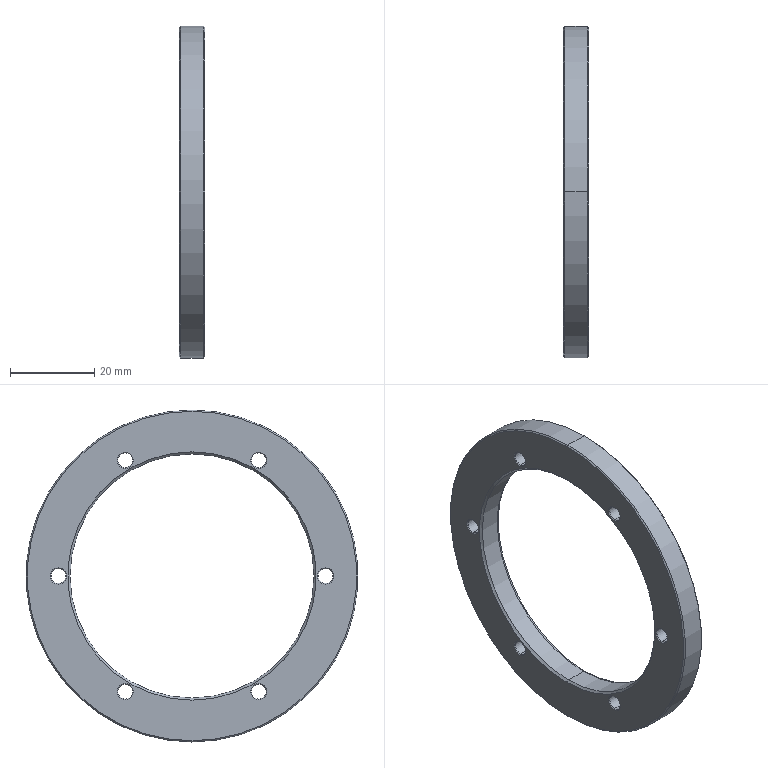Part | SolidWorks | features BaseBody 1 | 1 solid | 53 faces | box 6 x 78.9 x 78.9 mm | volume 13059 mm3 | cone 32 | cylinder 16 | plane 3 | torus 2 | commonest cylinder face diameters 3.5 x12 58 x2 78.9 x2
STEP:
#1=CARTESIAN_POINT('',(5.8,31.75,1.75));
#2=VERTEX_POINT('',#1);
#3=CARTESIAN_POINT('',(5.8,31.75,-1.75));
#4=VERTEX_POINT('',#3);
#5=CARTESIAN_POINT('',(5.8,31.75,0.));
#6=DIRECTION('',(1.,0.,0.));
#7=DIRECTION('',(0.,0.,1.));
#8=AXIS2_PLACEMENT_3D('',#5,#6,#7);
#9=CIRCLE('',#8,1.75);
#10=EDGE_CURVE('',#2,#4,#9,.T.);
#11=ORIENTED_EDGE('',*,*,#10,.F.);
#12=CARTESIAN_POINT('',(6.,31.75,1.95));
#13=VERTEX_POINT('',#12);
#14=CARTESIAN_POINT('',(6.,31.75,1.95));
#15=DIRECTION('',(0.7071,0.,0.7071));
#16=VECTOR('',#15,1000.);
#17=LINE('',#14,#16);
#18=EDGE_CURVE('',#2,#13,#17,.T.);
#19=ORIENTED_EDGE('',*,*,#18,.T.);
#20=CARTESIAN_POINT('',(6.,31.75,-1.95));
#21=VERTEX_POINT('',#20);
#22=CARTESIAN_POINT('',(6.,31.75,0.));
#23=DIRECTION('',(-1.,0.,0.));
#24=DIRECTION('',(0.,0.,1.));
#25=AXIS2_PLACEMENT_3D('',#22,#23,#24);
#26=CIRCLE('',#25,1.95);
#27=EDGE_CURVE('',#21,#13,#26,.T.);
#28=ORIENTED_EDGE('',*,*,#27,.F.);
#29=CARTESIAN_POINT('',(6.,31.75,-1.95));
#30=DIRECTION('',(0.7071,0.,-0.7071));
#31=VECTOR('',#30,1000.);
#32=LINE('',#29,#31);
#33=EDGE_CURVE('',#4,#21,#32,.T.);
#34=ORIENTED_EDGE('',*,*,#33,.F.);
#35=EDGE_LOOP('',(#11,#19,#28,#34));
#36=FACE_OUTER_BOUND('',#35,.T.);
#37=CARTESIAN_POINT('',(6.,31.75,0.));
#38=DIRECTION('',(1.,0.,0.));
#39=DIRECTION('',(0.,0.,-1.));
#40=AXIS2_PLACEMENT_3D('',#37,#38,#39);
#41=CONICAL_SURFACE('',#40,1.95,0.7854);
#42=ADVANCED_FACE('',(#36),#41,.F.);
#43=CARTESIAN_POINT('',(0.2,31.75,-1.75));
#44=VERTEX_POINT('',#43);
#45=CARTESIAN_POINT('',(0.2,31.75,1.75));
#46=VERTEX_POINT('',#45);
#47=CARTESIAN_POINT('',(0.2,31.75,0.));
#48=DIRECTION('',(-1.,0.,0.));
#49=DIRECTION('',(0.,0.,-1.));
#50=AXIS2_PLACEMENT_3D('',#47,#48,#49);
#51=CIRCLE('',#50,1.75);
#52=EDGE_CURVE('',#44,#46,#51,.T.);
#53=ORIENTED_EDGE('',*,*,#52,.F.);
#54=CARTESIAN_POINT('',(0.,31.75,-1.95));
#55=VERTEX_POINT('',#54);
#56=CARTESIAN_POINT('',(0.2,31.75,-1.75));
#57=DIRECTION('',(-0.7071,0.,-0.7071));
#58=VECTOR('',#57,1000.);
#59=LINE('',#56,#58);
#60=EDGE_CURVE('',#44,#55,#59,.T.);
#61=ORIENTED_EDGE('',*,*,#60,.T.);
#62=CARTESIAN_POINT('',(0.,31.75,1.95));
#63=VERTEX_POINT('',#62);
#64=CARTESIAN_POINT('',(0.,31.75,0.));
#65=DIRECTION('',(1.,0.,0.));
#66=DIRECTION('',(0.,0.,-1.));
#67=AXIS2_PLACEMENT_3D('',#64,#65,#66);
#68=CIRCLE('',#67,1.95);
#69=EDGE_CURVE('',#63,#55,#68,.T.);
#70=ORIENTED_EDGE('',*,*,#69,.F.);
#71=CARTESIAN_POINT('',(0.2,31.75,1.75));
#72=DIRECTION('',(-0.7071,0.,0.7071));
#73=VECTOR('',#72,1000.);
#74=LINE('',#71,#73);
#75=EDGE_CURVE('',#46,#63,#74,.T.);
#76=ORIENTED_EDGE('',*,*,#75,.F.);
#77=EDGE_LOOP('',(#53,#61,#70,#76));
#78=FACE_OUTER_BOUND('',#77,.T.);
#79=CARTESIAN_POINT('',(0.2,31.75,0.));
#80=DIRECTION('',(-1.,0.,0.));
#81=DIRECTION('',(0.,0.,1.));
#82=AXIS2_PLACEMENT_3D('',#79,#80,#81);
#83=CONICAL_SURFACE('',#82,1.75,0.7854);
#84=ADVANCED_FACE('',(#78),#83,.F.);
#85=CARTESIAN_POINT('',(5.8,15.875,-25.746));
#86=VERTEX_POINT('',#85);
#87=CARTESIAN_POINT('',(5.8,15.875,-29.246));
#88=VERTEX_POINT('',#87);
#89=CARTESIAN_POINT('',(5.8,15.875,-27.496));
#90=DIRECTION('',(1.,0.,0.));
#91=DIRECTION('',(0.,0.,1.));
#92=AXIS2_PLACEMENT_3D('',#89,#90,#91);
#93=CIRCLE('',#92,1.75);
#94=EDGE_CURVE('',#86,#88,#93,.T.);
#95=ORIENTED_EDGE('',*,*,#94,.F.);
#96=CARTESIAN_POINT('',(6.,15.875,-25.546));
#97=VERTEX_POINT('',#96);
#98=CARTESIAN_POINT('',(6.,15.875,-25.546));
#99=DIRECTION('',(0.7071,0.,0.7071));
#100=VECTOR('',#99,1000.);
#101=LINE('',#98,#100);
#102=EDGE_CURVE('',#86,#97,#101,.T.);
#103=ORIENTED_EDGE('',*,*,#102,.T.);
#104=CARTESIAN_POINT('',(6.,15.875,-29.446));
#105=VERTEX_POINT('',#104);
#106=CARTESIAN_POINT('',(6.,15.875,-27.496));
#107=DIRECTION('',(-1.,0.,0.));
#108=DIRECTION('',(0.,0.,1.));
#109=AXIS2_PLACEMENT_3D('',#106,#107,#108);
#110=CIRCLE('',#109,1.95);
#111=EDGE_CURVE('',#105,#97,#110,.T.);
#112=ORIENTED_EDGE('',*,*,#111,.F.);
#113=CARTESIAN_POINT('',(6.,15.875,-29.446));
#114=DIRECTION('',(0.7071,0.,-0.7071));
#115=VECTOR('',#114,1000.);
#116=LINE('',#113,#115);
#117=EDGE_CURVE('',#88,#105,#116,.T.);
#118=ORIENTED_EDGE('',*,*,#117,.F.);
#119=EDGE_LOOP('',(#95,#103,#112,#118));
#120=FACE_OUTER_BOUND('',#119,.T.);
#121=CARTESIAN_POINT('',(6.,15.875,-27.496));
#122=DIRECTION('',(1.,0.,0.));
#123=DIRECTION('',(0.,0.,-1.));
#124=AXIS2_PLACEMENT_3D('',#121,#122,#123);
#125=CONICAL_SURFACE('',#124,1.95,0.7854);
#126=ADVANCED_FACE('',(#120),#125,.F.);
#127=CARTESIAN_POINT('',(0.2,15.875,-29.246));
#128=VERTEX_POINT('',#127);
#129=CARTESIAN_POINT('',(0.2,15.875,-25.746));
#130=VERTEX_POINT('',#129);
#131=CARTESIAN_POINT('',(0.2,15.875,-27.496));
#132=DIRECTION('',(-1.,0.,0.));
#133=DIRECTION('',(0.,0.,-1.));
#134=AXIS2_PLACEMENT_3D('',#131,#132,#133);
#135=CIRCLE('',#134,1.75);
#136=EDGE_CURVE('',#128,#130,#135,.T.);
#137=ORIENTED_EDGE('',*,*,#136,.F.);
#138=CARTESIAN_POINT('',(0.,15.875,-29.446));
#139=VERTEX_POINT('',#138);
#140=CARTESIAN_POINT('',(0.2,15.875,-29.246));
#141=DIRECTION('',(-0.7071,0.,-0.7071));
#142=VECTOR('',#141,1000.);
#143=LINE('',#140,#142);
#144=EDGE_CURVE('',#128,#139,#143,.T.);
#145=ORIENTED_EDGE('',*,*,#144,.T.);
#146=CARTESIAN_POINT('',(0.,15.875,-25.546));
#147=VERTEX_POINT('',#146);
#148=CARTESIAN_POINT('',(0.,15.875,-27.496));
#149=DIRECTION('',(1.,0.,0.));
#150=DIRECTION('',(0.,0.,-1.));
#151=AXIS2_PLACEMENT_3D('',#148,#149,#150);
#152=CIRCLE('',#151,1.95);
#153=EDGE_CURVE('',#147,#139,#152,.T.);
#154=ORIENTED_EDGE('',*,*,#153,.F.);
#155=CARTESIAN_POINT('',(0.2,15.875,-25.746));
#156=DIRECTION('',(-0.7071,0.,0.7071));
#157=VECTOR('',#156,1000.);
#158=LINE('',#155,#157);
#159=EDGE_CURVE('',#130,#147,#158,.T.);
#160=ORIENTED_EDGE('',*,*,#159,.F.);
#161=EDGE_LOOP('',(#137,#145,#154,#160));
#162=FACE_OUTER_BOUND('',#161,.T.);
#163=CARTESIAN_POINT('',(0.2,15.875,-27.496));
#164=DIRECTION('',(-1.,0.,0.));
#165=DIRECTION('',(0.,0.,1.));
#166=AXIS2_PLACEMENT_3D('',#163,#164,#165);
#167=CONICAL_SURFACE('',#166,1.75,0.7854);
#168=ADVANCED_FACE('',(#162),#167,.F.);
#169=CARTESIAN_POINT('',(5.8,-15.875,-25.746));
#170=VERTEX_POINT('',#169);
#171=CARTESIAN_POINT('',(5.8,-15.875,-29.246));
#172=VERTEX_POINT('',#171);
#173=CARTESIAN_POINT('',(5.8,-15.875,-27.496));
#174=DIRECTION('',(1.,0.,0.));
#175=DIRECTION('',(0.,0.,1.));
#176=AXIS2_PLACEMENT_3D('',#173,#174,#175);
#177=CIRCLE('',#176,1.75);
#178=EDGE_CURVE('',#170,#172,#177,.T.);
#179=ORIENTED_EDGE('',*,*,#178,.F.);
#180=CARTESIAN_POINT('',(6.,-15.875,-25.546));
#181=VERTEX_POINT('',#180);
#182=CARTESIAN_POINT('',(6.,-15.875,-25.546));
#183=DIRECTION('',(0.7071,0.,0.7071));
#184=VECTOR('',#183,1000.);
#185=LINE('',#182,#184);
#186=EDGE_CURVE('',#170,#181,#185,.T.);
#187=ORIENTED_EDGE('',*,*,#186,.T.);
#188=CARTESIAN_POINT('',(6.,-15.875,-29.446));
#189=VERTEX_POINT('',#188);
#190=CARTESIAN_POINT('',(6.,-15.875,-27.496));
#191=DIRECTION('',(-1.,0.,0.));
#192=DIRECTION('',(0.,0.,1.));
#193=AXIS2_PLACEMENT_3D('',#190,#191,#192);
#194=CIRCLE('',#193,1.95);
#195=EDGE_CURVE('',#189,#181,#194,.T.);
#196=ORIENTED_EDGE('',*,*,#195,.F.);
#197=CARTESIAN_POINT('',(6.,-15.875,-29.446));
#198=DIRECTION('',(0.7071,0.,-0.7071));
#199=VECTOR('',#198,1000.);
#200=LINE('',#197,#199);
#201=EDGE_CURVE('',#172,#189,#200,.T.);
#202=ORIENTED_EDGE('',*,*,#201,.F.);
#203=EDGE_LOOP('',(#179,#187,#196,#202));
#204=FACE_OUTER_BOUND('',#203,.T.);
#205=CARTESIAN_POINT('',(6.,-15.875,-27.496));
#206=DIRECTION('',(1.,0.,0.));
#207=DIRECTION('',(0.,0.,-1.));
#208=AXIS2_PLACEMENT_3D('',#205,#206,#207);
#209=CONICAL_SURFACE('',#208,1.95,0.7854);
#210=ADVANCED_FACE('',(#204),#209,.F.);
#211=CARTESIAN_POINT('',(0.2,-15.875,-29.246));
#212=VERTEX_POINT('',#211);
#213=CARTESIAN_POINT('',(0.2,-15.875,-25.746));
#214=VERTEX_POINT('',#213);
#215=CARTESIAN_POINT('',(0.2,-15.875,-27.496));
#216=DIRECTION('',(-1.,0.,0.));
#217=DIRECTION('',(0.,0.,-1.));
#218=AXIS2_PLACEMENT_3D('',#215,#216,#217);
#219=CIRCLE('',#218,1.75);
#220=EDGE_CURVE('',#212,#214,#219,.T.);
#221=ORIENTED_EDGE('',*,*,#220,.F.);
#222=CARTESIAN_POINT('',(0.,-15.875,-29.446));
#223=VERTEX_POINT('',#222);
#224=CARTESIAN_POINT('',(0.2,-15.875,-29.246));
#225=DIRECTION('',(-0.7071,0.,-0.7071));
#226=VECTOR('',#225,1000.);
#227=LINE('',#224,#226);
#228=EDGE_CURVE('',#212,#223,#227,.T.);
#229=ORIENTED_EDGE('',*,*,#228,.T.);
#230=CARTESIAN_POINT('',(0.,-15.875,-25.546));
#231=VERTEX_POINT('',#230);
#232=CARTESIAN_POINT('',(0.,-15.875,-27.496));
#233=DIRECTION('',(1.,0.,0.));
#234=DIRECTION('',(0.,0.,-1.));
#235=AXIS2_PLACEMENT_3D('',#232,#233,#234);
#236=CIRCLE('',#235,1.95);
#237=EDGE_CURVE('',#231,#223,#236,.T.);
#238=ORIENTED_EDGE('',*,*,#237,.F.);
#239=CARTESIAN_POINT('',(0.2,-15.875,-25.746));
#240=DIRECTION('',(-0.7071,0.,0.7071));
#241=VECTOR('',#240,1000.);
#242=LINE('',#239,#241);
#243=EDGE_CURVE('',#214,#231,#242,.T.);
#244=ORIENTED_EDGE('',*,*,#243,.F.);
#245=EDGE_LOOP('',(#221,#229,#238,#244));
#246=FACE_OUTER_BOUND('',#245,.T.);
#247=CARTESIAN_POINT('',(0.2,-15.875,-27.496));
#248=DIRECTION('',(-1.,0.,0.));
#249=DIRECTION('',(0.,0.,1.));
#250=AXIS2_PLACEMENT_3D('',#247,#248,#249);
#251=CONICAL_SURFACE('',#250,1.75,0.7854);
#252=ADVANCED_FACE('',(#246),#251,.F.);
#253=CARTESIAN_POINT('',(5.8,-31.75,1.75));
#254=VERTEX_POINT('',#253);
#255=CARTESIAN_POINT('',(5.8,-31.75,-1.75));
#256=VERTEX_POINT('',#255);
#257=CARTESIAN_POINT('',(5.8,-31.75,0.));
#258=DIRECTION('',(1.,0.,0.));
#259=DIRECTION('',(0.,0.,1.));
#260=AXIS2_PLACEMENT_3D('',#257,#258,#259);
#261=CIRCLE('',#260,1.75);
#262=EDGE_CURVE('',#254,#256,#261,.T.);
#263=ORIENTED_EDGE('',*,*,#262,.F.);
#264=CARTESIAN_POINT('',(6.,-31.75,1.95));
#265=VERTEX_POINT('',#264);
#266=CARTESIAN_POINT('',(6.,-31.75,1.95));
#267=DIRECTION('',(0.7071,0.,0.7071));
#268=VECTOR('',#267,1000.);
#269=LINE('',#266,#268);
#270=EDGE_CURVE('',#254,#265,#269,.T.);
#271=ORIENTED_EDGE('',*,*,#270,.T.);
#272=CARTESIAN_POINT('',(6.,-31.75,-1.95));
#273=VERTEX_POINT('',#272);
#274=CARTESIAN_POINT('',(6.,-31.75,0.));
#275=DIRECTION('',(-1.,0.,0.));
#276=DIRECTION('',(0.,0.,1.));
#277=AXIS2_PLACEMENT_3D('',#274,#275,#276);
#278=CIRCLE('',#277,1.95);
#279=EDGE_CURVE('',#273,#265,#278,.T.);
#280=ORIENTED_EDGE('',*,*,#279,.F.);
#281=CARTESIAN_POINT('',(6.,-31.75,-1.95));
#282=DIRECTION('',(0.7071,0.,-0.7071));
#283=VECTOR('',#282,1000.);
#284=LINE('',#281,#283);
#285=EDGE_CURVE('',#256,#273,#284,.T.);
#286=ORIENTED_EDGE('',*,*,#285,.F.);
#287=EDGE_LOOP('',(#263,#271,#280,#286));
#288=FACE_OUTER_BOUND('',#287,.T.);
#289=CARTESIAN_POINT('',(6.,-31.75,0.));
#290=DIRECTION('',(1.,0.,0.));
#291=DIRECTION('',(0.,0.,-1.));
#292=AXIS2_PLACEMENT_3D('',#289,#290,#291);
#293=CONICAL_SURFACE('',#292,1.95,0.7854);
#294=ADVANCED_FACE('',(#288),#293,.F.);
#295=CARTESIAN_POINT('',(0.2,-31.75,-1.75));
#296=VERTEX_POINT('',#295);
#297=CARTESIAN_POINT('',(0.2,-31.75,1.75));
#298=VERTEX_POINT('',#297);
#299=CARTESIAN_POINT('',(0.2,-31.75,0.));
#300=DIRECTION('',(-1.,0.,0.));
#301=DIRECTION('',(0.,0.,-1.));
#302=AXIS2_PLACEMENT_3D('',#299,#300,#301);
#303=CIRCLE('',#302,1.75);
#304=EDGE_CURVE('',#296,#298,#303,.T.);
#305=ORIENTED_EDGE('',*,*,#304,.F.);
#306=CARTESIAN_POINT('',(0.,-31.75,-1.95));
#307=VERTEX_POINT('',#306);
#308=CARTESIAN_POINT('',(0.2,-31.75,-1.75));
#309=DIRECTION('',(-0.7071,0.,-0.7071));
#310=VECTOR('',#309,1000.);
#311=LINE('',#308,#310);
#312=EDGE_CURVE('',#296,#307,#311,.T.);
#313=ORIENTED_EDGE('',*,*,#312,.T.);
#314=CARTESIAN_POINT('',(0.,-31.75,1.95));
#315=VERTEX_POINT('',#314);
#316=CARTESIAN_POINT('',(0.,-31.75,0.));
#317=DIRECTION('',(1.,0.,0.));
#318=DIRECTION('',(0.,0.,-1.));
#319=AXIS2_PLACEMENT_3D('',#316,#317,#318);
#320=CIRCLE('',#319,1.95);
#321=EDGE_CURVE('',#315,#307,#320,.T.);
#322=ORIENTED_EDGE('',*,*,#321,.F.);
#323=CARTESIAN_POINT('',(0.2,-31.75,1.75));
#324=DIRECTION('',(-0.7071,0.,0.7071));
#325=VECTOR('',#324,1000.);
#326=LINE('',#323,#325);
#327=EDGE_CURVE('',#298,#315,#326,.T.);
#328=ORIENTED_EDGE('',*,*,#327,.F.);
#329=EDGE_LOOP('',(#305,#313,#322,#328));
#330=FACE_OUTER_BOUND('',#329,.T.);
#331=CARTESIAN_POINT('',(0.2,-31.75,0.));
#332=DIRECTION('',(-1.,0.,0.));
#333=DIRECTION('',(0.,0.,1.));
#334=AXIS2_PLACEMENT_3D('',#331,#332,#333);
#335=CONICAL_SURFACE('',#334,1.75,0.7854);
#336=ADVANCED_FACE('',(#330),#335,.F.);
#337=CARTESIAN_POINT('',(5.8,-15.875,29.246));
#338=VERTEX_POINT('',#337);
#339=CARTESIAN_POINT('',(5.8,-15.875,25.746));
#340=VERTEX_POINT('',#339);
#341=CARTESIAN_POINT('',(5.8,-15.875,27.496));
#342=DIRECTION('',(1.,0.,0.));
#343=DIRECTION('',(0.,0.,1.));
#344=AXIS2_PLACEMENT_3D('',#341,#342,#343);
#345=CIRCLE('',#344,1.75);
#346=EDGE_CURVE('',#338,#340,#345,.T.);
#347=ORIENTED_EDGE('',*,*,#346,.F.);
#348=CARTESIAN_POINT('',(6.,-15.875,29.446));
#349=VERTEX_POINT('',#348);
#350=CARTESIAN_POINT('',(6.,-15.875,29.446));
#351=DIRECTION('',(0.7071,0.,0.7071));
#352=VECTOR('',#351,1000.);
#353=LINE('',#350,#352);
#354=EDGE_CURVE('',#338,#349,#353,.T.);
#355=ORIENTED_EDGE('',*,*,#354,.T.);
#356=CARTESIAN_POINT('',(6.,-15.875,25.546));
#357=VERTEX_POINT('',#356);
#358=CARTESIAN_POINT('',(6.,-15.875,27.496));
#359=DIRECTION('',(-1.,0.,0.));
#360=DIRECTION('',(0.,0.,1.));
#361=AXIS2_PLACEMENT_3D('',#358,#359,#360);
#362=CIRCLE('',#361,1.95);
#363=EDGE_CURVE('',#357,#349,#362,.T.);
#364=ORIENTED_EDGE('',*,*,#363,.F.);
#365=CARTESIAN_POINT('',(6.,-15.875,25.546));
#366=DIRECTION('',(0.7071,0.,-0.7071));
#367=VECTOR('',#366,1000.);
#368=LINE('',#365,#367);
#369=EDGE_CURVE('',#340,#357,#368,.T.);
#370=ORIENTED_EDGE('',*,*,#369,.F.);
#371=EDGE_LOOP('',(#347,#355,#364,#370));
#372=FACE_OUTER_BOUND('',#371,.T.);
#373=CARTESIAN_POINT('',(6.,-15.875,27.496));
#374=DIRECTION('',(1.,0.,0.));
#375=DIRECTION('',(0.,0.,-1.));
#376=AXIS2_PLACEMENT_3D('',#373,#374,#375);
#377=CONICAL_SURFACE('',#376,1.95,0.7854);
#378=ADVANCED_FACE('',(#372),#377,.F.);
#379=CARTESIAN_POINT('',(0.2,-15.875,25.746));
#380=VERTEX_POINT('',#379);
#381=CARTESIAN_POINT('',(0.2,-15.875,29.246));
#382=VERTEX_POINT('',#381);
#383=CARTESIAN_POINT('',(0.2,-15.875,27.496));
#384=DIRECTION('',(-1.,0.,0.));
#385=DIRECTION('',(0.,0.,-1.));
#386=AXIS2_PLACEMENT_3D('',#383,#384,#385);
#387=CIRCLE('',#386,1.75);
#388=EDGE_CURVE('',#380,#382,#387,.T.);
#389=ORIENTED_EDGE('',*,*,#388,.F.);
#390=CARTESIAN_POINT('',(0.,-15.875,25.546));
#391=VERTEX_POINT('',#390);
#392=CARTESIAN_POINT('',(0.2,-15.875,25.746));
#393=DIRECTION('',(-0.7071,0.,-0.7071));
#394=VECTOR('',#393,1000.);
#395=LINE('',#392,#394);
#396=EDGE_CURVE('',#380,#391,#395,.T.);
#397=ORIENTED_EDGE('',*,*,#396,.T.);
#398=CARTESIAN_POINT('',(0.,-15.875,29.446));
#399=VERTEX_POINT('',#398);
#400=CARTESIAN_POINT('',(0.,-15.875,27.496));
#401=DIRECTION('',(1.,0.,0.));
#402=DIRECTION('',(0.,0.,-1.));
#403=AXIS2_PLACEMENT_3D('',#400,#401,#402);
#404=CIRCLE('',#403,1.95);
#405=EDGE_CURVE('',#399,#391,#404,.T.);
#406=ORIENTED_EDGE('',*,*,#405,.F.);
#407=CARTESIAN_POINT('',(0.2,-15.875,29.246));
#408=DIRECTION('',(-0.7071,0.,0.7071));
#409=VECTOR('',#408,1000.);
#410=LINE('',#407,#409);
#411=EDGE_CURVE('',#382,#399,#410,.T.);
#412=ORIENTED_EDGE('',*,*,#411,.F.);
#413=EDGE_LOOP('',(#389,#397,#406,#412));
#414=FACE_OUTER_BOUND('',#413,.T.);
#415=CARTESIAN_POINT('',(0.2,-15.875,27.496));
#416=DIRECTION('',(-1.,0.,0.));
#417=DIRECTION('',(0.,0.,1.));
#418=AXIS2_PLACEMENT_3D('',#415,#416,#417);
#419=CONICAL_SURFACE('',#418,1.75,0.7854);
#420=ADVANCED_FACE('',(#414),#419,.F.);
#421=CARTESIAN_POINT('',(5.8,15.875,29.246));
#422=VERTEX_POINT('',#421);
#423=CARTESIAN_POINT('',(5.8,15.875,25.746));
#424=VERTEX_POINT('',#423);
#425=CARTESIAN_POINT('',(5.8,15.875,27.496));
#426=DIRECTION('',(1.,0.,0.));
#427=DIRECTION('',(0.,0.,1.));
#428=AXIS2_PLACEMENT_3D('',#425,#426,#427);
#429=CIRCLE('',#428,1.75);
#430=EDGE_CURVE('',#422,#424,#429,.T.);
#431=ORIENTED_EDGE('',*,*,#430,.F.);
#432=CARTESIAN_POINT('',(6.,15.875,29.446));
#433=VERTEX_POINT('',#432);
#434=CARTESIAN_POINT('',(6.,15.875,29.446));
#435=DIRECTION('',(0.7071,0.,0.7071));
#436=VECTOR('',#435,1000.);
#437=LINE('',#434,#436);
#438=EDGE_CURVE('',#422,#433,#437,.T.);
#439=ORIENTED_EDGE('',*,*,#438,.T.);
#440=CARTESIAN_POINT('',(6.,15.875,25.546));
#441=VERTEX_POINT('',#440);
#442=CARTESIAN_POINT('',(6.,15.875,27.496));
#443=DIRECTION('',(-1.,0.,0.));
#444=DIRECTION('',(0.,0.,1.));
#445=AXIS2_PLACEMENT_3D('',#442,#443,#444);
#446=CIRCLE('',#445,1.95);
#447=EDGE_CURVE('',#441,#433,#446,.T.);
#448=ORIENTED_EDGE('',*,*,#447,.F.);
#449=CARTESIAN_POINT('',(6.,15.875,25.546));
#450=DIRECTION('',(0.7071,0.,-0.7071));
#451=VECTOR('',#450,1000.);
#452=LINE('',#449,#451);
#453=EDGE_CURVE('',#424,#441,#452,.T.);
#454=ORIENTED_EDGE('',*,*,#453,.F.);
#455=EDGE_LOOP('',(#431,#439,#448,#454));
#456=FACE_OUTER_BOUND('',#455,.T.);
#457=CARTESIAN_POINT('',(6.,15.875,27.496));
#458=DIRECTION('',(1.,0.,0.));
#459=DIRECTION('',(0.,0.,-1.));
#460=AXIS2_PLACEMENT_3D('',#457,#458,#459);
#461=CONICAL_SURFACE('',#460,1.95,0.7854);
#462=ADVANCED_FACE('',(#456),#461,.F.);
#463=CARTESIAN_POINT('',(0.2,15.875,25.746));
#464=VERTEX_POINT('',#463);
#465=CARTESIAN_POINT('',(0.2,15.875,29.246));
#466=VERTEX_POINT('',#465);
#467=CARTESIAN_POINT('',(0.2,15.875,27.496));
#468=DIRECTION('',(-1.,0.,0.));
#469=DIRECTION('',(0.,0.,-1.));
#470=AXIS2_PLACEMENT_3D('',#467,#468,#469);
#471=CIRCLE('',#470,1.75);
#472=EDGE_CURVE('',#464,#466,#471,.T.);
#473=ORIENTED_EDGE('',*,*,#472,.F.);
#474=CARTESIAN_POINT('',(0.,15.875,25.546));
#475=VERTEX_POINT('',#474);
#476=CARTESIAN_POINT('',(0.2,15.875,25.746));
#477=DIRECTION('',(-0.7071,0.,-0.7071));
#478=VECTOR('',#477,1000.);
#479=LINE('',#476,#478);
#480=EDGE_CURVE('',#464,#475,#479,.T.);
#481=ORIENTED_EDGE('',*,*,#480,.T.);
#482=CARTESIAN_POINT('',(0.,15.875,29.446));
#483=VERTEX_POINT('',#482);
#484=CARTESIAN_POINT('',(0.,15.875,27.496));
#485=DIRECTION('',(1.,0.,0.));
#486=DIRECTION('',(0.,0.,-1.));
#487=AXIS2_PLACEMENT_3D('',#484,#485,#486);
#488=CIRCLE('',#487,1.95);
#489=EDGE_CURVE('',#483,#475,#488,.T.);
#490=ORIENTED_EDGE('',*,*,#489,.F.);
#491=CARTESIAN_POINT('',(0.2,15.875,29.246));
#492=DIRECTION('',(-0.7071,0.,0.7071));
#493=VECTOR('',#492,1000.);
#494=LINE('',#491,#493);
#495=EDGE_CURVE('',#466,#483,#494,.T.);
#496=ORIENTED_EDGE('',*,*,#495,.F.);
#497=EDGE_LOOP('',(#473,#481,#490,#496));
#498=FACE_OUTER_BOUND('',#497,.T.);
#499=CARTESIAN_POINT('',(0.2,15.875,27.496));
#500=DIRECTION('',(-1.,0.,0.));
#501=DIRECTION('',(0.,0.,1.));
#502=AXIS2_PLACEMENT_3D('',#499,#500,#501);
#503=CONICAL_SURFACE('',#502,1.75,0.7854);
#504=ADVANCED_FACE('',(#498),#503,.F.);
#505=ORIENTED_EDGE('',*,*,#430,.T.);
#506=CARTESIAN_POINT('',(6.,15.875,25.746));
#507=DIRECTION('',(-1.,0.,0.));
#508=VECTOR('',#507,1000.);
#509=LINE('',#506,#508);
#510=EDGE_CURVE('',#424,#464,#509,.T.);
#511=ORIENTED_EDGE('',*,*,#510,.T.);
#512=ORIENTED_EDGE('',*,*,#472,.T.);
#513=CARTESIAN_POINT('',(6.,15.875,29.246));
#514=DIRECTION('',(-1.,0.,0.));
#515=VECTOR('',#514,1000.);
#516=LINE('',#513,#515);
#517=EDGE_CURVE('',#422,#466,#516,.T.);
#518=ORIENTED_EDGE('',*,*,#517,.F.);
#519=EDGE_LOOP('',(#505,#511,#512,#518));
#520=FACE_OUTER_BOUND('',#519,.T.);
#521=CARTESIAN_POINT('',(6.,15.875,27.496));
#522=DIRECTION('',(-1.,0.,0.));
#523=DIRECTION('',(0.,0.,1.));
#524=AXIS2_PLACEMENT_3D('',#521,#522,#523);
#525=CYLINDRICAL_SURFACE('',#524,1.75);
#526=ADVANCED_FACE('',(#520),#525,.F.);
#527=ORIENTED_EDGE('',*,*,#346,.T.);
#528=CARTESIAN_POINT('',(6.,-15.875,25.746));
#529=DIRECTION('',(-1.,0.,0.));
#530=VECTOR('',#529,1000.);
#531=LINE('',#528,#530);
#532=EDGE_CURVE('',#340,#380,#531,.T.);
#533=ORIENTED_EDGE('',*,*,#532,.T.);
#534=ORIENTED_EDGE('',*,*,#388,.T.);
#535=CARTESIAN_POINT('',(6.,-15.875,29.246));
#536=DIRECTION('',(-1.,0.,0.));
#537=VECTOR('',#536,1000.);
#538=LINE('',#535,#537);
#539=EDGE_CURVE('',#338,#382,#538,.T.);
#540=ORIENTED_EDGE('',*,*,#539,.F.);
#541=EDGE_LOOP('',(#527,#533,#534,#540));
#542=FACE_OUTER_BOUND('',#541,.T.);
#543=CARTESIAN_POINT('',(6.,-15.875,27.496));
#544=DIRECTION('',(-1.,0.,0.));
#545=DIRECTION('',(0.,0.,1.));
#546=AXIS2_PLACEMENT_3D('',#543,#544,#545);
#547=CYLINDRICAL_SURFACE('',#546,1.75);
#548=ADVANCED_FACE('',(#542),#547,.F.);
#549=ORIENTED_EDGE('',*,*,#262,.T.);
#550=CARTESIAN_POINT('',(6.,-31.75,-1.75));
#551=DIRECTION('',(-1.,0.,0.));
#552=VECTOR('',#551,1000.);
#553=LINE('',#550,#552);
#554=EDGE_CURVE('',#256,#296,#553,.T.);
#555=ORIENTED_EDGE('',*,*,#554,.T.);
#556=ORIENTED_EDGE('',*,*,#304,.T.);
#557=CARTESIAN_POINT('',(6.,-31.75,1.75));
#558=DIRECTION('',(-1.,0.,0.));
#559=VECTOR('',#558,1000.);
#560=LINE('',#557,#559);
#561=EDGE_CURVE('',#254,#298,#560,.T.);
#562=ORIENTED_EDGE('',*,*,#561,.F.);
#563=EDGE_LOOP('',(#549,#555,#556,#562));
#564=FACE_OUTER_BOUND('',#563,.T.);
#565=CARTESIAN_POINT('',(6.,-31.75,0.));
#566=DIRECTION('',(-1.,0.,0.));
#567=DIRECTION('',(0.,0.,1.));
#568=AXIS2_PLACEMENT_3D('',#565,#566,#567);
#569=CYLINDRICAL_SURFACE('',#568,1.75);
#570=ADVANCED_FACE('',(#564),#569,.F.);
#571=ORIENTED_EDGE('',*,*,#178,.T.);
#572=CARTESIAN_POINT('',(6.,-15.875,-29.246));
#573=DIRECTION('',(-1.,0.,0.));
#574=VECTOR('',#573,1000.);
#575=LINE('',#572,#574);
#576=EDGE_CURVE('',#172,#212,#575,.T.);
#577=ORIENTED_EDGE('',*,*,#576,.T.);
#578=ORIENTED_EDGE('',*,*,#220,.T.);
#579=CARTESIAN_POINT('',(6.,-15.875,-25.746));
#580=DIRECTION('',(-1.,0.,0.));
#581=VECTOR('',#580,1000.);
#582=LINE('',#579,#581);
#583=EDGE_CURVE('',#170,#214,#582,.T.);
#584=ORIENTED_EDGE('',*,*,#583,.F.);
#585=EDGE_LOOP('',(#571,#577,#578,#584));
#586=FACE_OUTER_BOUND('',#585,.T.);
#587=CARTESIAN_POINT('',(6.,-15.875,-27.496));
#588=DIRECTION('',(-1.,0.,0.));
#589=DIRECTION('',(0.,0.,1.));
#590=AXIS2_PLACEMENT_3D('',#587,#588,#589);
#591=CYLINDRICAL_SURFACE('',#590,1.75);
#592=ADVANCED_FACE('',(#586),#591,.F.);
#593=ORIENTED_EDGE('',*,*,#94,.T.);
#594=CARTESIAN_POINT('',(6.,15.875,-29.246));
#595=DIRECTION('',(-1.,0.,0.));
#596=VECTOR('',#595,1000.);
#597=LINE('',#594,#596);
#598=EDGE_CURVE('',#88,#128,#597,.T.);
#599=ORIENTED_EDGE('',*,*,#598,.T.);
#600=ORIENTED_EDGE('',*,*,#136,.T.);
#601=CARTESIAN_POINT('',(6.,15.875,-25.746));
#602=DIRECTION('',(-1.,0.,0.));
#603=VECTOR('',#602,1000.);
#604=LINE('',#601,#603);
#605=EDGE_CURVE('',#86,#130,#604,.T.);
#606=ORIENTED_EDGE('',*,*,#605,.F.);
#607=EDGE_LOOP('',(#593,#599,#600,#606));
#608=FACE_OUTER_BOUND('',#607,.T.);
#609=CARTESIAN_POINT('',(6.,15.875,-27.496));
#610=DIRECTION('',(-1.,0.,0.));
#611=DIRECTION('',(0.,0.,1.));
#612=AXIS2_PLACEMENT_3D('',#609,#610,#611);
#613=CYLINDRICAL_SURFACE('',#612,1.75);
#614=ADVANCED_FACE('',(#608),#613,.F.);
#615=ORIENTED_EDGE('',*,*,#10,.T.);
#616=CARTESIAN_POINT('',(6.,31.75,-1.75));
#617=DIRECTION('',(-1.,0.,0.));
#618=VECTOR('',#617,1000.);
#619=LINE('',#616,#618);
#620=EDGE_CURVE('',#4,#44,#619,.T.);
#621=ORIENTED_EDGE('',*,*,#620,.T.);
#622=ORIENTED_EDGE('',*,*,#52,.T.);
#623=CARTESIAN_POINT('',(6.,31.75,1.75));
#624=DIRECTION('',(-1.,0.,0.));
#625=VECTOR('',#624,1000.);
#626=LINE('',#623,#625);
#627=EDGE_CURVE('',#2,#46,#626,.T.);
#628=ORIENTED_EDGE('',*,*,#627,.F.);
#629=EDGE_LOOP('',(#615,#621,#622,#628));
#630=FACE_OUTER_BOUND('',#629,.T.);
#631=CARTESIAN_POINT('',(6.,31.75,0.));
#632=DIRECTION('',(-1.,0.,0.));
#633=DIRECTION('',(0.,0.,1.));
#634=AXIS2_PLACEMENT_3D('',#631,#632,#633);
#635=CYLINDRICAL_SURFACE('',#634,1.75);
#636=ADVANCED_FACE('',(#630),#635,.F.);
#637=CARTESIAN_POINT('',(0.5,0.,-29.));
#638=VERTEX_POINT('',#637);
#639=CARTESIAN_POINT('',(0.5,0.,29.));
#640=VERTEX_POINT('',#639);
#641=CARTESIAN_POINT('',(0.5,0.,0.));
#642=DIRECTION('',(-1.,0.,0.));
#643=DIRECTION('',(0.,0.,1.));
#644=AXIS2_PLACEMENT_3D('',#641,#642,#643);
#645=CIRCLE('',#644,29.);
#646=EDGE_CURVE('',#638,#640,#645,.T.);
#647=ORIENTED_EDGE('',*,*,#646,.F.);
#648=CARTESIAN_POINT('',(0.,0.,-29.5));
#649=VERTEX_POINT('',#648);
#650=CARTESIAN_POINT('',(0.,0.,-29.5));
#651=DIRECTION('',(-0.7071,0.,-0.7071));
#652=VECTOR('',#651,1000.);
#653=LINE('',#650,#652);
#654=EDGE_CURVE('',#638,#649,#653,.T.);
#655=ORIENTED_EDGE('',*,*,#654,.T.);
#656=CARTESIAN_POINT('',(0.,0.,29.5));
#657=VERTEX_POINT('',#656);
#658=CARTESIAN_POINT('',(0.,0.,0.));
#659=DIRECTION('',(-1.,0.,0.));
#660=DIRECTION('',(0.,0.,1.));
#661=AXIS2_PLACEMENT_3D('',#658,#659,#660);
#662=CIRCLE('',#661,29.5);
#663=EDGE_CURVE('',#649,#657,#662,.T.);
#664=ORIENTED_EDGE('',*,*,#663,.T.);
#665=CARTESIAN_POINT('',(0.,0.,29.5));
#666=DIRECTION('',(-0.7071,0.,0.7071));
#667=VECTOR('',#666,1000.);
#668=LINE('',#665,#667);
#669=EDGE_CURVE('',#640,#657,#668,.T.);
#670=ORIENTED_EDGE('',*,*,#669,.F.);
#671=EDGE_LOOP('',(#647,#655,#664,#670));
#672=FACE_OUTER_BOUND('',#671,.T.);
#673=CARTESIAN_POINT('',(0.,0.,0.));
#674=DIRECTION('',(-1.,0.,0.));
#675=DIRECTION('',(0.,0.,1.));
#676=AXIS2_PLACEMENT_3D('',#673,#674,#675);
#677=CONICAL_SURFACE('',#676,29.5,0.7854);
#678=ADVANCED_FACE('',(#672),#677,.F.);
#679=CARTESIAN_POINT('',(0.,0.,39.15));
#680=VERTEX_POINT('',#679);
#681=CARTESIAN_POINT('',(0.,0.,-39.15));
#682=VERTEX_POINT('',#681);
#683=CARTESIAN_POINT('',(0.,0.,0.));
#684=DIRECTION('',(-1.,0.,0.));
#685=DIRECTION('',(0.,0.,1.));
#686=AXIS2_PLACEMENT_3D('',#683,#684,#685);
#687=CIRCLE('',#686,39.15);
#688=EDGE_CURVE('',#680,#682,#687,.T.);
#689=ORIENTED_EDGE('',*,*,#688,.F.);
#690=CARTESIAN_POINT('',(0.3,0.,39.45));
#691=VERTEX_POINT('',#690);
#692=CARTESIAN_POINT('',(0.3,0.,39.45));
#693=DIRECTION('',(0.7071,0.,0.7071));
#694=VECTOR('',#693,1000.);
#695=LINE('',#692,#694);
#696=EDGE_CURVE('',#680,#691,#695,.T.);
#697=ORIENTED_EDGE('',*,*,#696,.T.);
#698=CARTESIAN_POINT('',(0.3,0.,-39.45));
#699=VERTEX_POINT('',#698);
#700=CARTESIAN_POINT('',(0.3,0.,0.));
#701=DIRECTION('',(-1.,0.,0.));
#702=DIRECTION('',(0.,0.,1.));
#703=AXIS2_PLACEMENT_3D('',#700,#701,#702);
#704=CIRCLE('',#703,39.45);
#705=EDGE_CURVE('',#691,#699,#704,.T.);
#706=ORIENTED_EDGE('',*,*,#705,.T.);
#707=CARTESIAN_POINT('',(0.3,0.,-39.45));
#708=DIRECTION('',(0.7071,0.,-0.7071));
#709=VECTOR('',#708,1000.);
#710=LINE('',#707,#709);
#711=EDGE_CURVE('',#682,#699,#710,.T.);
#712=ORIENTED_EDGE('',*,*,#711,.F.);
#713=EDGE_LOOP('',(#689,#697,#706,#712));
#714=FACE_OUTER_BOUND('',#713,.T.);
#715=CARTESIAN_POINT('',(0.3,0.,0.));
#716=DIRECTION('',(1.,0.,0.));
#717=DIRECTION('',(0.,0.,-1.));
#718=AXIS2_PLACEMENT_3D('',#715,#716,#717);
#719=CONICAL_SURFACE('',#718,39.45,0.7854);
#720=ADVANCED_FACE('',(#714),#719,.T.);
#721=CARTESIAN_POINT('',(5.7,0.,39.45));
#722=VERTEX_POINT('',#721);
#723=CARTESIAN_POINT('',(5.7,0.,-39.45));
#724=VERTEX_POINT('',#723);
#725=CARTESIAN_POINT('',(5.7,0.,0.));
#726=DIRECTION('',(-1.,0.,0.));
#727=DIRECTION('',(0.,0.,1.));
#728=AXIS2_PLACEMENT_3D('',#725,#726,#727);
#729=CIRCLE('',#728,39.45);
#730=EDGE_CURVE('',#722,#724,#729,.T.);
#731=ORIENTED_EDGE('',*,*,#730,.T.);
#732=CARTESIAN_POINT('',(0.,0.,-39.45));
#733=DIRECTION('',(-1.,0.,0.));
#734=VECTOR('',#733,1000.);
#735=LINE('',#732,#734);
#736=EDGE_CURVE('',#724,#699,#735,.T.);
#737=ORIENTED_EDGE('',*,*,#736,.T.);
#738=ORIENTED_EDGE('',*,*,#705,.F.);
#739=CARTESIAN_POINT('',(0.,0.,39.45));
#740=DIRECTION('',(-1.,0.,0.));
#741=VECTOR('',#740,1000.);
#742=LINE('',#739,#741);
#743=EDGE_CURVE('',#722,#691,#742,.T.);
#744=ORIENTED_EDGE('',*,*,#743,.F.);
#745=EDGE_LOOP('',(#731,#737,#738,#744));
#746=FACE_OUTER_BOUND('',#745,.T.);
#747=CARTESIAN_POINT('',(0.,0.,0.));
#748=DIRECTION('',(-1.,0.,0.));
#749=DIRECTION('',(0.,0.,1.));
#750=AXIS2_PLACEMENT_3D('',#747,#748,#749);
#751=CYLINDRICAL_SURFACE('',#750,39.45);
#752=ADVANCED_FACE('',(#746),#751,.T.);
#753=CARTESIAN_POINT('',(6.,0.,39.15));
#754=VERTEX_POINT('',#753);
#755=CARTESIAN_POINT('',(6.,0.,-39.15));
#756=VERTEX_POINT('',#755);
#757=CARTESIAN_POINT('',(6.,0.,0.));
#758=DIRECTION('',(-1.,0.,0.));
#759=DIRECTION('',(0.,0.,1.));
#760=AXIS2_PLACEMENT_3D('',#757,#758,#759);
#761=CIRCLE('',#760,39.15);
#762=EDGE_CURVE('',#754,#756,#761,.T.);
#763=ORIENTED_EDGE('',*,*,#762,.T.);
#764=CARTESIAN_POINT('',(6.,0.,-39.15));
#765=DIRECTION('',(-0.7071,0.,-0.7071));
#766=VECTOR('',#765,1000.);
#767=LINE('',#764,#766);
#768=EDGE_CURVE('',#756,#724,#767,.T.);
#769=ORIENTED_EDGE('',*,*,#768,.T.);
#770=ORIENTED_EDGE('',*,*,#730,.F.);
#771=CARTESIAN_POINT('',(6.,0.,39.15));
#772=DIRECTION('',(-0.7071,0.,0.7071));
#773=VECTOR('',#772,1000.);
#774=LINE('',#771,#773);
#775=EDGE_CURVE('',#754,#722,#774,.T.);
#776=ORIENTED_EDGE('',*,*,#775,.F.);
#777=EDGE_LOOP('',(#763,#769,#770,#776));
#778=FACE_OUTER_BOUND('',#777,.T.);
#779=CARTESIAN_POINT('',(6.,0.,0.));
#780=DIRECTION('',(-1.,0.,0.));
#781=DIRECTION('',(0.,0.,1.));
#782=AXIS2_PLACEMENT_3D('',#779,#780,#781);
#783=CONICAL_SURFACE('',#782,39.15,0.7854);
#784=ADVANCED_FACE('',(#778),#783,.T.);
#785=CARTESIAN_POINT('',(6.,0.,-35.346));
#786=VERTEX_POINT('',#785);
#787=CARTESIAN_POINT('',(6.,0.,35.346));
#788=VERTEX_POINT('',#787);
#789=CARTESIAN_POINT('',(6.,0.,0.));
#790=DIRECTION('',(-1.,0.,0.));
#791=DIRECTION('',(0.,0.,1.));
#792=AXIS2_PLACEMENT_3D('',#789,#790,#791);
#793=CIRCLE('',#792,35.346);
#794=EDGE_CURVE('',#786,#788,#793,.T.);
#795=ORIENTED_EDGE('',*,*,#794,.F.);
#796=CARTESIAN_POINT('',(6.,0.,-34.654));
#797=VERTEX_POINT('',#796);
#798=CARTESIAN_POINT('',(6.2,0.,-35.));
#799=DIRECTION('',(0.,1.,0.));
#800=DIRECTION('',(0.,0.,1.));
#801=AXIS2_PLACEMENT_3D('',#798,#799,#800);
#802=CIRCLE('',#801,0.4);
#803=EDGE_CURVE('',#786,#797,#802,.T.);
#804=ORIENTED_EDGE('',*,*,#803,.T.);
#805=CARTESIAN_POINT('',(6.,0.,34.654));
#806=VERTEX_POINT('',#805);
#807=CARTESIAN_POINT('',(6.,0.,0.));
#808=DIRECTION('',(-1.,0.,0.));
#809=DIRECTION('',(0.,0.,1.));
#810=AXIS2_PLACEMENT_3D('',#807,#808,#809);
#811=CIRCLE('',#810,34.654);
#812=EDGE_CURVE('',#797,#806,#811,.T.);
#813=ORIENTED_EDGE('',*,*,#812,.T.);
#814=CARTESIAN_POINT('',(6.2,0.,35.));
#815=DIRECTION('',(0.,-1.,0.));
#816=DIRECTION('',(0.,0.,-1.));
#817=AXIS2_PLACEMENT_3D('',#814,#815,#816);
#818=CIRCLE('',#817,0.4);
#819=EDGE_CURVE('',#788,#806,#818,.T.);
#820=ORIENTED_EDGE('',*,*,#819,.F.);
#821=EDGE_LOOP('',(#795,#804,#813,#820));
#822=FACE_OUTER_BOUND('',#821,.T.);
#823=CARTESIAN_POINT('',(6.2,0.,0.));
#824=DIRECTION('',(-1.,0.,0.));
#825=DIRECTION('',(0.,0.,1.));
#826=AXIS2_PLACEMENT_3D('',#823,#824,#825);
#827=TOROIDAL_SURFACE('',#826,35.,0.4);
#828=ADVANCED_FACE('',(#822),#827,.F.);
#829=CARTESIAN_POINT('',(5.5,0.,-29.));
#830=VERTEX_POINT('',#829);
#831=CARTESIAN_POINT('',(5.5,0.,29.));
#832=VERTEX_POINT('',#831);
#833=CARTESIAN_POINT('',(5.5,0.,0.));
#834=DIRECTION('',(-1.,0.,0.));
#835=DIRECTION('',(0.,0.,1.));
#836=AXIS2_PLACEMENT_3D('',#833,#834,#835);
#837=CIRCLE('',#836,29.);
#838=EDGE_CURVE('',#830,#832,#837,.T.);
#839=ORIENTED_EDGE('',*,*,#838,.T.);
#840=CARTESIAN_POINT('',(6.,0.,29.182));
#841=VERTEX_POINT('',#840);
#842=CARTESIAN_POINT('',(5.5,0.,29.));
#843=DIRECTION('',(0.9397,0.,0.342));
#844=VECTOR('',#843,1000.);
#845=LINE('',#842,#844);
#846=EDGE_CURVE('',#832,#841,#845,.T.);
#847=ORIENTED_EDGE('',*,*,#846,.T.);
#848=CARTESIAN_POINT('',(6.,0.,-29.182));
#849=VERTEX_POINT('',#848);
#850=CARTESIAN_POINT('',(6.,0.,0.));
#851=DIRECTION('',(-1.,0.,0.));
#852=DIRECTION('',(0.,0.,1.));
#853=AXIS2_PLACEMENT_3D('',#850,#851,#852);
#854=CIRCLE('',#853,29.182);
#855=EDGE_CURVE('',#849,#841,#854,.T.);
#856=ORIENTED_EDGE('',*,*,#855,.F.);
#857=CARTESIAN_POINT('',(5.5,0.,-29.));
#858=DIRECTION('',(0.9397,0.,-0.342));
#859=VECTOR('',#858,1000.);
#860=LINE('',#857,#859);
#861=EDGE_CURVE('',#830,#849,#860,.T.);
#862=ORIENTED_EDGE('',*,*,#861,.F.);
#863=EDGE_LOOP('',(#839,#847,#856,#862));
#864=FACE_OUTER_BOUND('',#863,.T.);
#865=CARTESIAN_POINT('',(5.5,0.,0.));
#866=DIRECTION('',(1.,0.,0.));
#867=DIRECTION('',(0.,0.,-1.));
#868=AXIS2_PLACEMENT_3D('',#865,#866,#867);
#869=CONICAL_SURFACE('',#868,29.,0.3491);
#870=ADVANCED_FACE('',(#864),#869,.F.);
#871=ORIENTED_EDGE('',*,*,#838,.F.);
#872=CARTESIAN_POINT('',(0.,0.,-29.));
#873=DIRECTION('',(-1.,0.,0.));
#874=VECTOR('',#873,1000.);
#875=LINE('',#872,#874);
#876=EDGE_CURVE('',#830,#638,#875,.T.);
#877=ORIENTED_EDGE('',*,*,#876,.T.);
#878=ORIENTED_EDGE('',*,*,#646,.T.);
#879=CARTESIAN_POINT('',(0.,0.,29.));
#880=DIRECTION('',(-1.,0.,0.));
#881=VECTOR('',#880,1000.);
#882=LINE('',#879,#881);
#883=EDGE_CURVE('',#832,#640,#882,.T.);
#884=ORIENTED_EDGE('',*,*,#883,.F.);
#885=EDGE_LOOP('',(#871,#877,#878,#884));
#886=FACE_OUTER_BOUND('',#885,.T.);
#887=CARTESIAN_POINT('',(0.,0.,0.));
#888=DIRECTION('',(-1.,0.,0.));
#889=DIRECTION('',(0.,0.,1.));
#890=AXIS2_PLACEMENT_3D('',#887,#888,#889);
#891=CYLINDRICAL_SURFACE('',#890,29.);
#892=ADVANCED_FACE('',(#886),#891,.F.);
#893=ORIENTED_EDGE('',*,*,#876,.F.);
#894=CARTESIAN_POINT('',(5.5,0.,0.));
#895=DIRECTION('',(-1.,0.,0.));
#896=DIRECTION('',(0.,0.,1.));
#897=AXIS2_PLACEMENT_3D('',#894,#895,#896);
#898=CIRCLE('',#897,29.);
#899=EDGE_CURVE('',#832,#830,#898,.T.);
#900=ORIENTED_EDGE('',*,*,#899,.F.);
#901=ORIENTED_EDGE('',*,*,#883,.T.);
#902=CARTESIAN_POINT('',(0.5,0.,0.));
#903=DIRECTION('',(-1.,0.,0.));
#904=DIRECTION('',(0.,0.,1.));
#905=AXIS2_PLACEMENT_3D('',#902,#903,#904);
#906=CIRCLE('',#905,29.);
#907=EDGE_CURVE('',#640,#638,#906,.T.);
#908=ORIENTED_EDGE('',*,*,#907,.T.);
#909=EDGE_LOOP('',(#893,#900,#901,#908));
#910=FACE_OUTER_BOUND('',#909,.T.);
#911=CARTESIAN_POINT('',(0.,0.,0.));
#912=DIRECTION('',(-1.,0.,0.));
#913=DIRECTION('',(0.,0.,1.));
#914=AXIS2_PLACEMENT_3D('',#911,#912,#913);
#915=CYLINDRICAL_SURFACE('',#914,29.);
#916=ADVANCED_FACE('',(#910),#915,.F.);
#917=ORIENTED_EDGE('',*,*,#846,.F.);
#918=ORIENTED_EDGE('',*,*,#899,.T.);
#919=ORIENTED_EDGE('',*,*,#861,.T.);
#920=CARTESIAN_POINT('',(6.,0.,0.));
#921=DIRECTION('',(-1.,0.,0.));
#922=DIRECTION('',(0.,0.,1.));
#923=AXIS2_PLACEMENT_3D('',#920,#921,#922);
#924=CIRCLE('',#923,29.182);
#925=EDGE_CURVE('',#841,#849,#924,.T.);
#926=ORIENTED_EDGE('',*,*,#925,.F.);
#927=EDGE_LOOP('',(#917,#918,#919,#926));
#928=FACE_OUTER_BOUND('',#927,.T.);
#929=CARTESIAN_POINT('',(5.5,0.,0.));
#930=DIRECTION('',(1.,0.,0.));
#931=DIRECTION('',(0.,0.,-1.));
#932=AXIS2_PLACEMENT_3D('',#929,#930,#931);
#933=CONICAL_SURFACE('',#932,29.,0.3491);
#934=ADVANCED_FACE('',(#928),#933,.F.);
#935=ORIENTED_EDGE('',*,*,#447,.T.);
#936=CARTESIAN_POINT('',(6.,15.875,27.496));
#937=DIRECTION('',(-1.,0.,0.));
#938=DIRECTION('',(0.,0.,1.));
#939=AXIS2_PLACEMENT_3D('',#936,#937,#938);
#940=CIRCLE('',#939,1.95);
#941=EDGE_CURVE('',#433,#441,#940,.T.);
#942=ORIENTED_EDGE('',*,*,#941,.T.);
#943=EDGE_LOOP('',(#935,#942));
#944=FACE_BOUND('',#943,.T.);
#945=ORIENTED_EDGE('',*,*,#363,.T.);
#946=CARTESIAN_POINT('',(6.,-15.875,27.496));
#947=DIRECTION('',(-1.,0.,0.));
#948=DIRECTION('',(0.,0.,1.));
#949=AXIS2_PLACEMENT_3D('',#946,#947,#948);
#950=CIRCLE('',#949,1.95);
#951=EDGE_CURVE('',#349,#357,#950,.T.);
#952=ORIENTED_EDGE('',*,*,#951,.T.);
#953=EDGE_LOOP('',(#945,#952));
#954=FACE_BOUND('',#953,.T.);
#955=ORIENTED_EDGE('',*,*,#279,.T.);
#956=CARTESIAN_POINT('',(6.,-31.75,0.));
#957=DIRECTION('',(-1.,0.,0.));
#958=DIRECTION('',(0.,0.,1.));
#959=AXIS2_PLACEMENT_3D('',#956,#957,#958);
#960=CIRCLE('',#959,1.95);
#961=EDGE_CURVE('',#265,#273,#960,.T.);
#962=ORIENTED_EDGE('',*,*,#961,.T.);
#963=EDGE_LOOP('',(#955,#962));
#964=FACE_BOUND('',#963,.T.);
#965=ORIENTED_EDGE('',*,*,#195,.T.);
#966=CARTESIAN_POINT('',(6.,-15.875,-27.496));
#967=DIRECTION('',(-1.,0.,0.));
#968=DIRECTION('',(0.,0.,1.));
#969=AXIS2_PLACEMENT_3D('',#966,#967,#968);
#970=CIRCLE('',#969,1.95);
#971=EDGE_CURVE('',#181,#189,#970,.T.);
#972=ORIENTED_EDGE('',*,*,#971,.T.);
#973=EDGE_LOOP('',(#965,#972));
#974=FACE_BOUND('',#973,.T.);
#975=ORIENTED_EDGE('',*,*,#111,.T.);
#976=CARTESIAN_POINT('',(6.,15.875,-27.496));
#977=DIRECTION('',(-1.,0.,0.));
#978=DIRECTION('',(0.,0.,1.));
#979=AXIS2_PLACEMENT_3D('',#976,#977,#978);
#980=CIRCLE('',#979,1.95);
#981=EDGE_CURVE('',#97,#105,#980,.T.);
#982=ORIENTED_EDGE('',*,*,#981,.T.);
#983=EDGE_LOOP('',(#975,#982));
#984=FACE_BOUND('',#983,.T.);
#985=ORIENTED_EDGE('',*,*,#27,.T.);
#986=CARTESIAN_POINT('',(6.,31.75,0.));
#987=DIRECTION('',(-1.,0.,0.));
#988=DIRECTION('',(0.,0.,1.));
#989=AXIS2_PLACEMENT_3D('',#986,#987,#988);
#990=CIRCLE('',#989,1.95);
#991=EDGE_CURVE('',#13,#21,#990,.T.);
#992=ORIENTED_EDGE('',*,*,#991,.T.);
#993=EDGE_LOOP('',(#985,#992));
#994=FACE_BOUND('',#993,.T.);
#995=ORIENTED_EDGE('',*,*,#855,.T.);
#996=ORIENTED_EDGE('',*,*,#925,.T.);
#997=EDGE_LOOP('',(#995,#996));
#998=FACE_BOUND('',#997,.T.);
#999=CARTESIAN_POINT('',(6.,0.,0.));
#1000=DIRECTION('',(-1.,0.,0.));
#1001=DIRECTION('',(0.,0.,1.));
#1002=AXIS2_PLACEMENT_3D('',#999,#1000,#1001);
#1003=CIRCLE('',#1002,34.654);
#1004=EDGE_CURVE('',#806,#797,#1003,.T.);
#1005=ORIENTED_EDGE('',*,*,#1004,.F.);
#1006=ORIENTED_EDGE('',*,*,#812,.F.);
#1007=EDGE_LOOP('',(#1005,#1006));
#1008=FACE_OUTER_BOUND('',#1007,.T.);
#1009=CARTESIAN_POINT('',(6.,34.654,0.));
#1010=DIRECTION('',(-1.,0.,0.));
#1011=DIRECTION('',(0.,0.,1.));
#1012=AXIS2_PLACEMENT_3D('',#1009,#1010,#1011);
#1013=PLANE('',#1012);
#1014=ADVANCED_FACE('',(#944,#954,#964,#974,#984,#994,#998,#1008),#1013,.F.);
#1015=ORIENTED_EDGE('',*,*,#803,.F.);
#1016=CARTESIAN_POINT('',(6.,0.,0.));
#1017=DIRECTION('',(-1.,0.,0.));
#1018=DIRECTION('',(0.,0.,1.));
#1019=AXIS2_PLACEMENT_3D('',#1016,#1017,#1018);
#1020=CIRCLE('',#1019,35.346);
#1021=EDGE_CURVE('',#788,#786,#1020,.T.);
#1022=ORIENTED_EDGE('',*,*,#1021,.F.);
#1023=ORIENTED_EDGE('',*,*,#819,.T.);
#1024=ORIENTED_EDGE('',*,*,#1004,.T.);
#1025=EDGE_LOOP('',(#1015,#1022,#1023,#1024));
#1026=FACE_OUTER_BOUND('',#1025,.T.);
#1027=CARTESIAN_POINT('',(6.2,0.,0.));
#1028=DIRECTION('',(-1.,0.,0.));
#1029=DIRECTION('',(0.,0.,1.));
#1030=AXIS2_PLACEMENT_3D('',#1027,#1028,#1029);
#1031=TOROIDAL_SURFACE('',#1030,35.,0.4);
#1032=ADVANCED_FACE('',(#1026),#1031,.F.);
#1033=ORIENTED_EDGE('',*,*,#1021,.T.);
#1034=ORIENTED_EDGE('',*,*,#794,.T.);
#1035=EDGE_LOOP('',(#1033,#1034));
#1036=FACE_BOUND('',#1035,.T.);
#1037=ORIENTED_EDGE('',*,*,#762,.F.);
#1038=CARTESIAN_POINT('',(6.,0.,0.));
#1039=DIRECTION('',(-1.,0.,0.));
#1040=DIRECTION('',(0.,0.,1.));
#1041=AXIS2_PLACEMENT_3D('',#1038,#1039,#1040);
#1042=CIRCLE('',#1041,39.15);
#1043=EDGE_CURVE('',#756,#754,#1042,.T.);
#1044=ORIENTED_EDGE('',*,*,#1043,.F.);
#1045=EDGE_LOOP('',(#1037,#1044));
#1046=FACE_OUTER_BOUND('',#1045,.T.);
#1047=CARTESIAN_POINT('',(6.,39.15,0.));
#1048=DIRECTION('',(-1.,0.,0.));
#1049=DIRECTION('',(0.,0.,1.));
#1050=AXIS2_PLACEMENT_3D('',#1047,#1048,#1049);
#1051=PLANE('',#1050);
#1052=ADVANCED_FACE('',(#1036,#1046),#1051,.F.);
#1053=ORIENTED_EDGE('',*,*,#768,.F.);
#1054=ORIENTED_EDGE('',*,*,#1043,.T.);
#1055=ORIENTED_EDGE('',*,*,#775,.T.);
#1056=CARTESIAN_POINT('',(5.7,0.,0.));
#1057=DIRECTION('',(-1.,0.,0.));
#1058=DIRECTION('',(0.,0.,1.));
#1059=AXIS2_PLACEMENT_3D('',#1056,#1057,#1058);
#1060=CIRCLE('',#1059,39.45);
#1061=EDGE_CURVE('',#724,#722,#1060,.T.);
#1062=ORIENTED_EDGE('',*,*,#1061,.F.);
#1063=EDGE_LOOP('',(#1053,#1054,#1055,#1062));
#1064=FACE_OUTER_BOUND('',#1063,.T.);
#1065=CARTESIAN_POINT('',(6.,0.,0.));
#1066=DIRECTION('',(-1.,0.,0.));
#1067=DIRECTION('',(0.,0.,1.));
#1068=AXIS2_PLACEMENT_3D('',#1065,#1066,#1067);
#1069=CONICAL_SURFACE('',#1068,39.15,0.7854);
#1070=ADVANCED_FACE('',(#1064),#1069,.T.);
#1071=ORIENTED_EDGE('',*,*,#736,.F.);
#1072=ORIENTED_EDGE('',*,*,#1061,.T.);
#1073=ORIENTED_EDGE('',*,*,#743,.T.);
#1074=CARTESIAN_POINT('',(0.3,0.,0.));
#1075=DIRECTION('',(-1.,0.,0.));
#1076=DIRECTION('',(0.,0.,1.));
#1077=AXIS2_PLACEMENT_3D('',#1074,#1075,#1076);
#1078=CIRCLE('',#1077,39.45);
#1079=EDGE_CURVE('',#699,#691,#1078,.T.);
#1080=ORIENTED_EDGE('',*,*,#1079,.F.);
#1081=EDGE_LOOP('',(#1071,#1072,#1073,#1080));
#1082=FACE_OUTER_BOUND('',#1081,.T.);
#1083=CARTESIAN_POINT('',(0.,0.,0.));
#1084=DIRECTION('',(-1.,0.,0.));
#1085=DIRECTION('',(0.,0.,1.));
#1086=AXIS2_PLACEMENT_3D('',#1083,#1084,#1085);
#1087=CYLINDRICAL_SURFACE('',#1086,39.45);
#1088=ADVANCED_FACE('',(#1082),#1087,.T.);
#1089=ORIENTED_EDGE('',*,*,#696,.F.);
#1090=CARTESIAN_POINT('',(0.,0.,0.));
#1091=DIRECTION('',(-1.,0.,0.));
#1092=DIRECTION('',(0.,0.,1.));
#1093=AXIS2_PLACEMENT_3D('',#1090,#1091,#1092);
#1094=CIRCLE('',#1093,39.15);
#1095=EDGE_CURVE('',#682,#680,#1094,.T.);
#1096=ORIENTED_EDGE('',*,*,#1095,.F.);
#1097=ORIENTED_EDGE('',*,*,#711,.T.);
#1098=ORIENTED_EDGE('',*,*,#1079,.T.);
#1099=EDGE_LOOP('',(#1089,#1096,#1097,#1098));
#1100=FACE_OUTER_BOUND('',#1099,.T.);
#1101=CARTESIAN_POINT('',(0.3,0.,0.));
#1102=DIRECTION('',(1.,0.,0.));
#1103=DIRECTION('',(0.,0.,-1.));
#1104=AXIS2_PLACEMENT_3D('',#1101,#1102,#1103);
#1105=CONICAL_SURFACE('',#1104,39.45,0.7854);
#1106=ADVANCED_FACE('',(#1100),#1105,.T.);
#1107=ORIENTED_EDGE('',*,*,#489,.T.);
#1108=CARTESIAN_POINT('',(0.,15.875,27.496));
#1109=DIRECTION('',(1.,0.,0.));
#1110=DIRECTION('',(0.,0.,-1.));
#1111=AXIS2_PLACEMENT_3D('',#1108,#1109,#1110);
#1112=CIRCLE('',#1111,1.95);
#1113=EDGE_CURVE('',#475,#483,#1112,.T.);
#1114=ORIENTED_EDGE('',*,*,#1113,.T.);
#1115=EDGE_LOOP('',(#1107,#1114));
#1116=FACE_BOUND('',#1115,.T.);
#1117=ORIENTED_EDGE('',*,*,#405,.T.);
#1118=CARTESIAN_POINT('',(0.,-15.875,27.496));
#1119=DIRECTION('',(1.,0.,0.));
#1120=DIRECTION('',(0.,0.,-1.));
#1121=AXIS2_PLACEMENT_3D('',#1118,#1119,#1120);
#1122=CIRCLE('',#1121,1.95);
#1123=EDGE_CURVE('',#391,#399,#1122,.T.);
#1124=ORIENTED_EDGE('',*,*,#1123,.T.);
#1125=EDGE_LOOP('',(#1117,#1124));
#1126=FACE_BOUND('',#1125,.T.);
#1127=ORIENTED_EDGE('',*,*,#321,.T.);
#1128=CARTESIAN_POINT('',(0.,-31.75,0.));
#1129=DIRECTION('',(1.,0.,0.));
#1130=DIRECTION('',(0.,0.,-1.));
#1131=AXIS2_PLACEMENT_3D('',#1128,#1129,#1130);
#1132=CIRCLE('',#1131,1.95);
#1133=EDGE_CURVE('',#307,#315,#1132,.T.);
#1134=ORIENTED_EDGE('',*,*,#1133,.T.);
#1135=EDGE_LOOP('',(#1127,#1134));
#1136=FACE_BOUND('',#1135,.T.);
#1137=ORIENTED_EDGE('',*,*,#237,.T.);
#1138=CARTESIAN_POINT('',(0.,-15.875,-27.496));
#1139=DIRECTION('',(1.,0.,0.));
#1140=DIRECTION('',(0.,0.,-1.));
#1141=AXIS2_PLACEMENT_3D('',#1138,#1139,#1140);
#1142=CIRCLE('',#1141,1.95);
#1143=EDGE_CURVE('',#223,#231,#1142,.T.);
#1144=ORIENTED_EDGE('',*,*,#1143,.T.);
#1145=EDGE_LOOP('',(#1137,#1144));
#1146=FACE_BOUND('',#1145,.T.);
#1147=ORIENTED_EDGE('',*,*,#153,.T.);
#1148=CARTESIAN_POINT('',(0.,15.875,-27.496));
#1149=DIRECTION('',(1.,0.,0.));
#1150=DIRECTION('',(0.,0.,-1.));
#1151=AXIS2_PLACEMENT_3D('',#1148,#1149,#1150);
#1152=CIRCLE('',#1151,1.95);
#1153=EDGE_CURVE('',#139,#147,#1152,.T.);
#1154=ORIENTED_EDGE('',*,*,#1153,.T.);
#1155=EDGE_LOOP('',(#1147,#1154));
#1156=FACE_BOUND('',#1155,.T.);
#1157=ORIENTED_EDGE('',*,*,#69,.T.);
#1158=CARTESIAN_POINT('',(0.,31.75,0.));
#1159=DIRECTION('',(1.,0.,0.));
#1160=DIRECTION('',(0.,0.,-1.));
#1161=AXIS2_PLACEMENT_3D('',#1158,#1159,#1160);
#1162=CIRCLE('',#1161,1.95);
#1163=EDGE_CURVE('',#55,#63,#1162,.T.);
#1164=ORIENTED_EDGE('',*,*,#1163,.T.);
#1165=EDGE_LOOP('',(#1157,#1164));
#1166=FACE_BOUND('',#1165,.T.);
#1167=CARTESIAN_POINT('',(0.,0.,0.));
#1168=DIRECTION('',(-1.,0.,0.));
#1169=DIRECTION('',(0.,0.,1.));
#1170=AXIS2_PLACEMENT_3D('',#1167,#1168,#1169);
#1171=CIRCLE('',#1170,29.5);
#1172=EDGE_CURVE('',#657,#649,#1171,.T.);
#1173=ORIENTED_EDGE('',*,*,#1172,.F.);
#1174=ORIENTED_EDGE('',*,*,#663,.F.);
#1175=EDGE_LOOP('',(#1173,#1174));
#1176=FACE_BOUND('',#1175,.T.);
#1177=ORIENTED_EDGE('',*,*,#1095,.T.);
#1178=ORIENTED_EDGE('',*,*,#688,.T.);
#1179=EDGE_LOOP('',(#1177,#1178));
#1180=FACE_OUTER_BOUND('',#1179,.T.);
#1181=CARTESIAN_POINT('',(0.,39.15,0.));
#1182=DIRECTION('',(1.,0.,0.));
#1183=DIRECTION('',(0.,1.,0.));
#1184=AXIS2_PLACEMENT_3D('',#1181,#1182,#1183);
#1185=PLANE('',#1184);
#1186=ADVANCED_FACE('',(#1116,#1126,#1136,#1146,#1156,#1166,#1176,#1180),#1185,.F.);
#1187=ORIENTED_EDGE('',*,*,#654,.F.);
#1188=ORIENTED_EDGE('',*,*,#907,.F.);
#1189=ORIENTED_EDGE('',*,*,#669,.T.);
#1190=ORIENTED_EDGE('',*,*,#1172,.T.);
#1191=EDGE_LOOP('',(#1187,#1188,#1189,#1190));
#1192=FACE_OUTER_BOUND('',#1191,.T.);
#1193=CARTESIAN_POINT('',(0.,0.,0.));
#1194=DIRECTION('',(-1.,0.,0.));
#1195=DIRECTION('',(0.,0.,1.));
#1196=AXIS2_PLACEMENT_3D('',#1193,#1194,#1195);
#1197=CONICAL_SURFACE('',#1196,29.5,0.7854);
#1198=ADVANCED_FACE('',(#1192),#1197,.F.);
#1199=ORIENTED_EDGE('',*,*,#620,.F.);
#1200=CARTESIAN_POINT('',(5.8,31.75,0.));
#1201=DIRECTION('',(1.,0.,0.));
#1202=DIRECTION('',(0.,0.,1.));
#1203=AXIS2_PLACEMENT_3D('',#1200,#1201,#1202);
#1204=CIRCLE('',#1203,1.75);
#1205=EDGE_CURVE('',#4,#2,#1204,.T.);
#1206=ORIENTED_EDGE('',*,*,#1205,.T.);
#1207=ORIENTED_EDGE('',*,*,#627,.T.);
#1208=CARTESIAN_POINT('',(0.2,31.75,0.));
#1209=DIRECTION('',(-1.,0.,0.));
#1210=DIRECTION('',(0.,0.,-1.));
#1211=AXIS2_PLACEMENT_3D('',#1208,#1209,#1210);
#1212=CIRCLE('',#1211,1.75);
#1213=EDGE_CURVE('',#46,#44,#1212,.T.);
#1214=ORIENTED_EDGE('',*,*,#1213,.T.);
#1215=EDGE_LOOP('',(#1199,#1206,#1207,#1214));
#1216=FACE_OUTER_BOUND('',#1215,.T.);
#1217=CARTESIAN_POINT('',(6.,31.75,0.));
#1218=DIRECTION('',(-1.,0.,0.));
#1219=DIRECTION('',(0.,0.,1.));
#1220=AXIS2_PLACEMENT_3D('',#1217,#1218,#1219);
#1221=CYLINDRICAL_SURFACE('',#1220,1.75);
#1222=ADVANCED_FACE('',(#1216),#1221,.F.);
#1223=ORIENTED_EDGE('',*,*,#598,.F.);
#1224=CARTESIAN_POINT('',(5.8,15.875,-27.496));
#1225=DIRECTION('',(1.,0.,0.));
#1226=DIRECTION('',(0.,0.,1.));
#1227=AXIS2_PLACEMENT_3D('',#1224,#1225,#1226);
#1228=CIRCLE('',#1227,1.75);
#1229=EDGE_CURVE('',#88,#86,#1228,.T.);
#1230=ORIENTED_EDGE('',*,*,#1229,.T.);
#1231=ORIENTED_EDGE('',*,*,#605,.T.);
#1232=CARTESIAN_POINT('',(0.2,15.875,-27.496));
#1233=DIRECTION('',(-1.,0.,0.));
#1234=DIRECTION('',(0.,0.,-1.));
#1235=AXIS2_PLACEMENT_3D('',#1232,#1233,#1234);
#1236=CIRCLE('',#1235,1.75);
#1237=EDGE_CURVE('',#130,#128,#1236,.T.);
#1238=ORIENTED_EDGE('',*,*,#1237,.T.);
#1239=EDGE_LOOP('',(#1223,#1230,#1231,#1238));
#1240=FACE_OUTER_BOUND('',#1239,.T.);
#1241=CARTESIAN_POINT('',(6.,15.875,-27.496));
#1242=DIRECTION('',(-1.,0.,0.));
#1243=DIRECTION('',(0.,0.,1.));
#1244=AXIS2_PLACEMENT_3D('',#1241,#1242,#1243);
#1245=CYLINDRICAL_SURFACE('',#1244,1.75);
#1246=ADVANCED_FACE('',(#1240),#1245,.F.);
#1247=ORIENTED_EDGE('',*,*,#576,.F.);
#1248=CARTESIAN_POINT('',(5.8,-15.875,-27.496));
#1249=DIRECTION('',(1.,0.,0.));
#1250=DIRECTION('',(0.,0.,1.));
#1251=AXIS2_PLACEMENT_3D('',#1248,#1249,#1250);
#1252=CIRCLE('',#1251,1.75);
#1253=EDGE_CURVE('',#172,#170,#1252,.T.);
#1254=ORIENTED_EDGE('',*,*,#1253,.T.);
#1255=ORIENTED_EDGE('',*,*,#583,.T.);
#1256=CARTESIAN_POINT('',(0.2,-15.875,-27.496));
#1257=DIRECTION('',(-1.,0.,0.));
#1258=DIRECTION('',(0.,0.,-1.));
#1259=AXIS2_PLACEMENT_3D('',#1256,#1257,#1258);
#1260=CIRCLE('',#1259,1.75);
#1261=EDGE_CURVE('',#214,#212,#1260,.T.);
#1262=ORIENTED_EDGE('',*,*,#1261,.T.);
#1263=EDGE_LOOP('',(#1247,#1254,#1255,#1262));
#1264=FACE_OUTER_BOUND('',#1263,.T.);
#1265=CARTESIAN_POINT('',(6.,-15.875,-27.496));
#1266=DIRECTION('',(-1.,0.,0.));
#1267=DIRECTION('',(0.,0.,1.));
#1268=AXIS2_PLACEMENT_3D('',#1265,#1266,#1267);
#1269=CYLINDRICAL_SURFACE('',#1268,1.75);
#1270=ADVANCED_FACE('',(#1264),#1269,.F.);
#1271=ORIENTED_EDGE('',*,*,#554,.F.);
#1272=CARTESIAN_POINT('',(5.8,-31.75,0.));
#1273=DIRECTION('',(1.,0.,0.));
#1274=DIRECTION('',(0.,0.,1.));
#1275=AXIS2_PLACEMENT_3D('',#1272,#1273,#1274);
#1276=CIRCLE('',#1275,1.75);
#1277=EDGE_CURVE('',#256,#254,#1276,.T.);
#1278=ORIENTED_EDGE('',*,*,#1277,.T.);
#1279=ORIENTED_EDGE('',*,*,#561,.T.);
#1280=CARTESIAN_POINT('',(0.2,-31.75,0.));
#1281=DIRECTION('',(-1.,0.,0.));
#1282=DIRECTION('',(0.,0.,-1.));
#1283=AXIS2_PLACEMENT_3D('',#1280,#1281,#1282);
#1284=CIRCLE('',#1283,1.75);
#1285=EDGE_CURVE('',#298,#296,#1284,.T.);
#1286=ORIENTED_EDGE('',*,*,#1285,.T.);
#1287=EDGE_LOOP('',(#1271,#1278,#1279,#1286));
#1288=FACE_OUTER_BOUND('',#1287,.T.);
#1289=CARTESIAN_POINT('',(6.,-31.75,0.));
#1290=DIRECTION('',(-1.,0.,0.));
#1291=DIRECTION('',(0.,0.,1.));
#1292=AXIS2_PLACEMENT_3D('',#1289,#1290,#1291);
#1293=CYLINDRICAL_SURFACE('',#1292,1.75);
#1294=ADVANCED_FACE('',(#1288),#1293,.F.);
#1295=ORIENTED_EDGE('',*,*,#532,.F.);
#1296=CARTESIAN_POINT('',(5.8,-15.875,27.496));
#1297=DIRECTION('',(1.,0.,0.));
#1298=DIRECTION('',(0.,0.,1.));
#1299=AXIS2_PLACEMENT_3D('',#1296,#1297,#1298);
#1300=CIRCLE('',#1299,1.75);
#1301=EDGE_CURVE('',#340,#338,#1300,.T.);
#1302=ORIENTED_EDGE('',*,*,#1301,.T.);
#1303=ORIENTED_EDGE('',*,*,#539,.T.);
#1304=CARTESIAN_POINT('',(0.2,-15.875,27.496));
#1305=DIRECTION('',(-1.,0.,0.));
#1306=DIRECTION('',(0.,0.,-1.));
#1307=AXIS2_PLACEMENT_3D('',#1304,#1305,#1306);
#1308=CIRCLE('',#1307,1.75);
#1309=EDGE_CURVE('',#382,#380,#1308,.T.);
#1310=ORIENTED_EDGE('',*,*,#1309,.T.);
#1311=EDGE_LOOP('',(#1295,#1302,#1303,#1310));
#1312=FACE_OUTER_BOUND('',#1311,.T.);
#1313=CARTESIAN_POINT('',(6.,-15.875,27.496));
#1314=DIRECTION('',(-1.,0.,0.));
#1315=DIRECTION('',(0.,0.,1.));
#1316=AXIS2_PLACEMENT_3D('',#1313,#1314,#1315);
#1317=CYLINDRICAL_SURFACE('',#1316,1.75);
#1318=ADVANCED_FACE('',(#1312),#1317,.F.);
#1319=ORIENTED_EDGE('',*,*,#510,.F.);
#1320=CARTESIAN_POINT('',(5.8,15.875,27.496));
#1321=DIRECTION('',(1.,0.,0.));
#1322=DIRECTION('',(0.,0.,1.));
#1323=AXIS2_PLACEMENT_3D('',#1320,#1321,#1322);
#1324=CIRCLE('',#1323,1.75);
#1325=EDGE_CURVE('',#424,#422,#1324,.T.);
#1326=ORIENTED_EDGE('',*,*,#1325,.T.);
#1327=ORIENTED_EDGE('',*,*,#517,.T.);
#1328=CARTESIAN_POINT('',(0.2,15.875,27.496));
#1329=DIRECTION('',(-1.,0.,0.));
#1330=DIRECTION('',(0.,0.,-1.));
#1331=AXIS2_PLACEMENT_3D('',#1328,#1329,#1330);
#1332=CIRCLE('',#1331,1.75);
#1333=EDGE_CURVE('',#466,#464,#1332,.T.);
#1334=ORIENTED_EDGE('',*,*,#1333,.T.);
#1335=EDGE_LOOP('',(#1319,#1326,#1327,#1334));
#1336=FACE_OUTER_BOUND('',#1335,.T.);
#1337=CARTESIAN_POINT('',(6.,15.875,27.496));
#1338=DIRECTION('',(-1.,0.,0.));
#1339=DIRECTION('',(0.,0.,1.));
#1340=AXIS2_PLACEMENT_3D('',#1337,#1338,#1339);
#1341=CYLINDRICAL_SURFACE('',#1340,1.75);
#1342=ADVANCED_FACE('',(#1336),#1341,.F.);
#1343=ORIENTED_EDGE('',*,*,#480,.F.);
#1344=ORIENTED_EDGE('',*,*,#1333,.F.);
#1345=ORIENTED_EDGE('',*,*,#495,.T.);
#1346=ORIENTED_EDGE('',*,*,#1113,.F.);
#1347=EDGE_LOOP('',(#1343,#1344,#1345,#1346));
#1348=FACE_OUTER_BOUND('',#1347,.T.);
#1349=CARTESIAN_POINT('',(0.2,15.875,27.496));
#1350=DIRECTION('',(-1.,0.,0.));
#1351=DIRECTION('',(0.,0.,1.));
#1352=AXIS2_PLACEMENT_3D('',#1349,#1350,#1351);
#1353=CONICAL_SURFACE('',#1352,1.75,0.7854);
#1354=ADVANCED_FACE('',(#1348),#1353,.F.);
#1355=ORIENTED_EDGE('',*,*,#438,.F.);
#1356=ORIENTED_EDGE('',*,*,#1325,.F.);
#1357=ORIENTED_EDGE('',*,*,#453,.T.);
#1358=ORIENTED_EDGE('',*,*,#941,.F.);
#1359=EDGE_LOOP('',(#1355,#1356,#1357,#1358));
#1360=FACE_OUTER_BOUND('',#1359,.T.);
#1361=CARTESIAN_POINT('',(6.,15.875,27.496));
#1362=DIRECTION('',(1.,0.,0.));
#1363=DIRECTION('',(0.,0.,-1.));
#1364=AXIS2_PLACEMENT_3D('',#1361,#1362,#1363);
#1365=CONICAL_SURFACE('',#1364,1.95,0.7854);
#1366=ADVANCED_FACE('',(#1360),#1365,.F.);
#1367=ORIENTED_EDGE('',*,*,#396,.F.);
#1368=ORIENTED_EDGE('',*,*,#1309,.F.);
#1369=ORIENTED_EDGE('',*,*,#411,.T.);
#1370=ORIENTED_EDGE('',*,*,#1123,.F.);
#1371=EDGE_LOOP('',(#1367,#1368,#1369,#1370));
#1372=FACE_OUTER_BOUND('',#1371,.T.);
#1373=CARTESIAN_POINT('',(0.2,-15.875,27.496));
#1374=DIRECTION('',(-1.,0.,0.));
#1375=DIRECTION('',(0.,0.,1.));
#1376=AXIS2_PLACEMENT_3D('',#1373,#1374,#1375);
#1377=CONICAL_SURFACE('',#1376,1.75,0.7854);
#1378=ADVANCED_FACE('',(#1372),#1377,.F.);
#1379=ORIENTED_EDGE('',*,*,#354,.F.);
#1380=ORIENTED_EDGE('',*,*,#1301,.F.);
#1381=ORIENTED_EDGE('',*,*,#369,.T.);
#1382=ORIENTED_EDGE('',*,*,#951,.F.);
#1383=EDGE_LOOP('',(#1379,#1380,#1381,#1382));
#1384=FACE_OUTER_BOUND('',#1383,.T.);
#1385=CARTESIAN_POINT('',(6.,-15.875,27.496));
#1386=DIRECTION('',(1.,0.,0.));
#1387=DIRECTION('',(0.,0.,-1.));
#1388=AXIS2_PLACEMENT_3D('',#1385,#1386,#1387);
#1389=CONICAL_SURFACE('',#1388,1.95,0.7854);
#1390=ADVANCED_FACE('',(#1384),#1389,.F.);
#1391=ORIENTED_EDGE('',*,*,#312,.F.);
#1392=ORIENTED_EDGE('',*,*,#1285,.F.);
#1393=ORIENTED_EDGE('',*,*,#327,.T.);
#1394=ORIENTED_EDGE('',*,*,#1133,.F.);
#1395=EDGE_LOOP('',(#1391,#1392,#1393,#1394));
#1396=FACE_OUTER_BOUND('',#1395,.T.);
#1397=CARTESIAN_POINT('',(0.2,-31.75,0.));
#1398=DIRECTION('',(-1.,0.,0.));
#1399=DIRECTION('',(0.,0.,1.));
#1400=AXIS2_PLACEMENT_3D('',#1397,#1398,#1399);
#1401=CONICAL_SURFACE('',#1400,1.75,0.7854);
#1402=ADVANCED_FACE('',(#1396),#1401,.F.);
#1403=ORIENTED_EDGE('',*,*,#270,.F.);
#1404=ORIENTED_EDGE('',*,*,#1277,.F.);
#1405=ORIENTED_EDGE('',*,*,#285,.T.);
#1406=ORIENTED_EDGE('',*,*,#961,.F.);
#1407=EDGE_LOOP('',(#1403,#1404,#1405,#1406));
#1408=FACE_OUTER_BOUND('',#1407,.T.);
#1409=CARTESIAN_POINT('',(6.,-31.75,0.));
#1410=DIRECTION('',(1.,0.,0.));
#1411=DIRECTION('',(0.,0.,-1.));
#1412=AXIS2_PLACEMENT_3D('',#1409,#1410,#1411);
#1413=CONICAL_SURFACE('',#1412,1.95,0.7854);
#1414=ADVANCED_FACE('',(#1408),#1413,.F.);
#1415=ORIENTED_EDGE('',*,*,#228,.F.);
#1416=ORIENTED_EDGE('',*,*,#1261,.F.);
#1417=ORIENTED_EDGE('',*,*,#243,.T.);
#1418=ORIENTED_EDGE('',*,*,#1143,.F.);
#1419=EDGE_LOOP('',(#1415,#1416,#1417,#1418));
#1420=FACE_OUTER_BOUND('',#1419,.T.);
#1421=CARTESIAN_POINT('',(0.2,-15.875,-27.496));
#1422=DIRECTION('',(-1.,0.,0.));
#1423=DIRECTION('',(0.,0.,1.));
#1424=AXIS2_PLACEMENT_3D('',#1421,#1422,#1423);
#1425=CONICAL_SURFACE('',#1424,1.75,0.7854);
#1426=ADVANCED_FACE('',(#1420),#1425,.F.);
#1427=ORIENTED_EDGE('',*,*,#186,.F.);
#1428=ORIENTED_EDGE('',*,*,#1253,.F.);
#1429=ORIENTED_EDGE('',*,*,#201,.T.);
#1430=ORIENTED_EDGE('',*,*,#971,.F.);
#1431=EDGE_LOOP('',(#1427,#1428,#1429,#1430));
#1432=FACE_OUTER_BOUND('',#1431,.T.);
#1433=CARTESIAN_POINT('',(6.,-15.875,-27.496));
#1434=DIRECTION('',(1.,0.,0.));
#1435=DIRECTION('',(0.,0.,-1.));
#1436=AXIS2_PLACEMENT_3D('',#1433,#1434,#1435);
#1437=CONICAL_SURFACE('',#1436,1.95,0.7854);
#1438=ADVANCED_FACE('',(#1432),#1437,.F.);
#1439=ORIENTED_EDGE('',*,*,#144,.F.);
#1440=ORIENTED_EDGE('',*,*,#1237,.F.);
#1441=ORIENTED_EDGE('',*,*,#159,.T.);
#1442=ORIENTED_EDGE('',*,*,#1153,.F.);
#1443=EDGE_LOOP('',(#1439,#1440,#1441,#1442));
#1444=FACE_OUTER_BOUND('',#1443,.T.);
#1445=CARTESIAN_POINT('',(0.2,15.875,-27.496));
#1446=DIRECTION('',(-1.,0.,0.));
#1447=DIRECTION('',(0.,0.,1.));
#1448=AXIS2_PLACEMENT_3D('',#1445,#1446,#1447);
#1449=CONICAL_SURFACE('',#1448,1.75,0.7854);
#1450=ADVANCED_FACE('',(#1444),#1449,.F.);
#1451=ORIENTED_EDGE('',*,*,#102,.F.);
#1452=ORIENTED_EDGE('',*,*,#1229,.F.);
#1453=ORIENTED_EDGE('',*,*,#117,.T.);
#1454=ORIENTED_EDGE('',*,*,#981,.F.);
#1455=EDGE_LOOP('',(#1451,#1452,#1453,#1454));
#1456=FACE_OUTER_BOUND('',#1455,.T.);
#1457=CARTESIAN_POINT('',(6.,15.875,-27.496));
#1458=DIRECTION('',(1.,0.,0.));
#1459=DIRECTION('',(0.,0.,-1.));
#1460=AXIS2_PLACEMENT_3D('',#1457,#1458,#1459);
#1461=CONICAL_SURFACE('',#1460,1.95,0.7854);
#1462=ADVANCED_FACE('',(#1456),#1461,.F.);
#1463=ORIENTED_EDGE('',*,*,#60,.F.);
#1464=ORIENTED_EDGE('',*,*,#1213,.F.);
#1465=ORIENTED_EDGE('',*,*,#75,.T.);
#1466=ORIENTED_EDGE('',*,*,#1163,.F.);
#1467=EDGE_LOOP('',(#1463,#1464,#1465,#1466));
#1468=FACE_OUTER_BOUND('',#1467,.T.);
#1469=CARTESIAN_POINT('',(0.2,31.75,0.));
#1470=DIRECTION('',(-1.,0.,0.));
#1471=DIRECTION('',(0.,0.,1.));
#1472=AXIS2_PLACEMENT_3D('',#1469,#1470,#1471);
#1473=CONICAL_SURFACE('',#1472,1.75,0.7854);
#1474=ADVANCED_FACE('',(#1468),#1473,.F.);
#1475=ORIENTED_EDGE('',*,*,#18,.F.);
#1476=ORIENTED_EDGE('',*,*,#1205,.F.);
#1477=ORIENTED_EDGE('',*,*,#33,.T.);
#1478=ORIENTED_EDGE('',*,*,#991,.F.);
#1479=EDGE_LOOP('',(#1475,#1476,#1477,#1478));
#1480=FACE_OUTER_BOUND('',#1479,.T.);
#1481=CARTESIAN_POINT('',(6.,31.75,0.));
#1482=DIRECTION('',(1.,0.,0.));
#1483=DIRECTION('',(0.,0.,-1.));
#1484=AXIS2_PLACEMENT_3D('',#1481,#1482,#1483);
#1485=CONICAL_SURFACE('',#1484,1.95,0.7854);
#1486=ADVANCED_FACE('',(#1480),#1485,.F.);
#1487=CLOSED_SHELL('',(#42,#84,#126,#168,#210,#252,#294,#336,#378,#420,#462,#504,#526,#548,#570,#592,#614,#636,#678,#720,#752,#784,#828,#870,#892,#916,#934,#1014,#1032,#1052,#1070,#1088,#1106,#1186,#1198,#1222,#1246,#1270,#1294,#1318,#1342,#1354,#1366,#1378,#1390,#1402,#1414,#1426,#1438,#1450,#1462,#1474,#1486));
#1488=MANIFOLD_SOLID_BREP('',#1487);
#1489=CARTESIAN_POINT('',(0.,0.,0.));
#1490=DIRECTION('',(0.,0.,1.));
#1491=DIRECTION('',(1.,0.,0.));
#1492=AXIS2_PLACEMENT_3D('',#1489,#1490,#1491);
#1493=(LENGTH_UNIT()NAMED_UNIT(*)SI_UNIT(.MILLI.,.METRE.));
#1494=UNCERTAINTY_MEASURE_WITH_UNIT(LENGTH_MEASURE(0.00001),#1493,'','');
#1495=(NAMED_UNIT(*)PLANE_ANGLE_UNIT()SI_UNIT($,.RADIAN.));
#1496=(NAMED_UNIT(*)SI_UNIT($,.STERADIAN.)SOLID_ANGLE_UNIT());
#1497=(GEOMETRIC_REPRESENTATION_CONTEXT(3)GLOBAL_UNCERTAINTY_ASSIGNED_CONTEXT((#1494))GLOBAL_UNIT_ASSIGNED_CONTEXT((#1493,#1495,#1496))REPRESENTATION_CONTEXT('',''));
#1498=ADVANCED_BREP_SHAPE_REPRESENTATION('',(#1488,#1492),#1497);